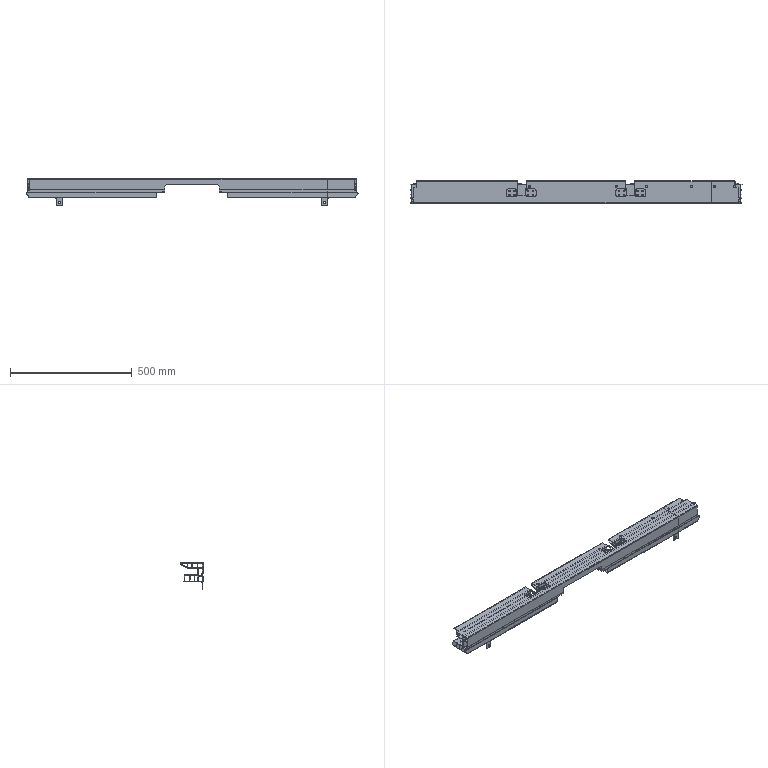NC program | NX | posted with a generic post | part box 1365 x 90.95 x 108.501 mm
Lines 9781 to 10665 of 25066:
(ZLEVEL_PROFILE_1_COPY_1_1 , TOOL : D8R0.5)
N19530 T08 M6
N19532 G54
N19534 G17 G0 G90 X660.495 Y57.439 B0. C0. S6000 M3
N19536 G43 Z30. H8
N19538 Z-42.865
N19540 G94 G1 Z-44.365 F1000.
N19542 X660.199 Y56.252
N19544 G3 X660.42 Y55.483 R0.8
N19546 G1 X660.758 Y55.156 F2500.
N19548 X662.222 Y53.696
N19550 X662.428 Y53.488
N19552 G3 X666.413 Y49.491 R729.531
N19554 G1 X666.616 Y49.475
N19556 Z-44.465
N19558 X666.413 Y49.491
N19560 G2 X663.219 Y52.689 R774.294
N19562 G1 X663.021 Y52.89
N19564 X660.715 Y55.202
N19566 X660.417 Y55.487
N19568 X660.418 Z-44.565
N19570 G2 X663.021 Y52.89 R195.375
N19572 G3 X666.414 Y49.491 R625.386
N19574 G1 X666.616 Y49.475
N19576 Z-44.665
N19578 X666.415 Y49.491
N19580 X665.211 Y50.69
N19582 X665.018 Y50.876
N19584 X664.809 Y51.09
N19586 X661.445 Y54.478
N19588 G3 X660.419 Y55.488 R64.335
N19590 G1 X660.42 Z-44.765
N19592 G2 X660.72 Y55.196 R23.551
N19594 X665.018 Y50.878 R530.21
N19596 G1 X665.214 Y50.69
N19598 X666.419 Y49.491
N19600 X666.616 Y49.475
N19602 Z-44.865
N19604 X666.425 Y49.491
N19606 X664.811 Y51.09
N19608 X664.619 Y51.282
N19610 G3 X663.021 Y52.891 R113.024
N19612 X661.024 Y54.894 R137.528
N19614 X660.421 Y55.489 R22.994
N19616 G1 X660.422 Y55.49 Z-44.965
N19618 G2 X661.024 Y54.899 R23.36
N19620 X663.021 Y52.892 R119.536
N19622 X664.619 Y51.286 R86.72
N19624 G1 X664.816 Y51.09
N19626 X666.431 Y49.491
N19628 X666.616 Y49.475
N19630 Z-45.064
N19632 X666.437 Y49.491
N19634 X666.217 Y49.713
N19636 X665.018 Y50.889
N19638 G3 X662.834 Y53.088 R301.433
N19640 X660.424 Y55.492 R93.733
N19642 G1 X660.442 Y55.478 Z-45.163
N19644 G2 X663.021 Y52.901 R125.339
N19646 X664.619 Y51.294 R58.969
N19648 G1 X664.824 Y51.09
N19650 X666.217 Y49.718
N19652 X666.443 Y49.491
N19654 X666.616 Y49.475
N19656 Z-45.262
N19658 X666.451 Y49.491
N19660 G3 X664.619 Y51.299 R214.938
N19662 X663.021 Y52.905 R42.782
N19664 X660.466 Y55.459 R115.023
N19666 G1 X660.504 Y55.426 Z-45.362
N19668 G2 X663.021 Y52.914 R106.424
N19670 X664.619 Y51.31 R47.085
N19672 G1 X666.463 Y49.491
N19674 X666.616 Y49.475
N19676 Z-45.462
N19678 X666.475 Y49.491
N19680 G3 X664.619 Y51.322 R957.072
N19682 X663.021 Y52.925 R54.744
N19684 X661.265 Y54.687 R80.824
N19686 G1 X660.547 Y55.392
N19688 X660.53 Y55.405
N19690 X660.554 Y55.39 Z-45.562
N19692 X660.869 Y55.087
N19694 X662.622 Y53.345
N19696 X663.021 Y52.936
N19698 G2 X664.862 Y51.09 R94.393
N19700 G1 X666.49 Y49.491
N19702 X666.616 Y49.475
N19704 Z-45.662
N19706 X666.508 Y49.491
N19708 G3 X664.872 Y51.09 R406.168
N19710 X660.587 Y55.368 R402.037
N19712 G1 X660.61 Y55.355 Z-45.762
N19714 G2 X665.285 Y50.69 R543.174
N19716 X666.525 Y49.491 R40.797
N19718 G1 X666.616 Y49.475
N19720 Z-45.862
N19722 X666.543 Y49.491
N19724 G3 X665.302 Y50.69 R40.86
N19726 G1 X664.895 Y51.09
N19728 G3 X663.299 Y52.689 R54.249
N19730 G1 X662.905 Y53.088
N19732 X660.747 Y55.232
N19734 X660.644 Y55.332
N19736 X660.674 Y55.313 Z-45.962
N19738 X664.529 Y51.49
N19740 X664.619 Y51.392
N19742 G3 X665.817 Y50.223 R29.773
N19744 G1 X666.56 Y49.491
N19746 X666.616 Y49.475
N19748 Z-46.062
N19750 X666.578 Y49.491
N19752 X665.817 Y50.239
N19754 G2 X664.619 Y51.411 R31.256
N19756 G1 X664.546 Y51.49
N19758 G2 X660.704 Y55.294 R6488.3
N19760 G1 X660.732 Y55.276 Z-46.162
N19762 X663.82 Y52.221
N19764 X664.563 Y51.49
N19766 G3 X665.779 Y50.291 R30.069
N19768 G1 X665.817 Y50.255
N19770 X666.595 Y49.491
N19772 X666.616 Y49.475
N19774 X667.016 Z-46.262
N19776 X666.616 Y49.488
N19778 X665.797 Y50.291
N19780 G2 X664.58 Y51.49 R32.969
N19782 X660.762 Y55.258 R1601.449
N19784 G1 X660.797 Y55.233 Z-46.362
N19786 G2 X665.418 Y50.67 R1621.061
N19788 G1 X666.64 Y49.491
N19790 X667.016 Y49.475
N19792 Z-46.462
N19794 X666.669 Y49.491
N19796 X665.415 Y50.69
N19798 G3 X660.823 Y55.217 R862.367
N19800 G1 X660.856 Y55.203 Z-46.562
N19802 G2 X665.442 Y50.69 R2264.451
N19804 G1 X666.699 Y49.491
N19806 X667.016 Y49.475
N19808 Z-46.662
N19810 X666.728 Y49.491
N19812 X665.418 Y50.741
N19814 G3 X660.888 Y55.188 R10000.
N19816 G1 X660.921 Y55.173 Z-46.762
N19818 X663.86 Y52.289
N19820 X664.219 Y51.946
N19822 G3 X666.758 Y49.491 R134.499
N19824 G1 X667.016 Y49.475
N19826 Z-46.862
N19828 X666.787 Y49.491
N19830 G2 X664.219 Y51.969 R138.511
N19832 G1 X663.879 Y52.289
N19834 X660.954 Y55.158
N19836 X660.987 Y55.144 Z-46.962
N19838 X661.024 Y55.109
N19840 X663.421 Y52.753
N19842 X663.898 Y52.289
N19844 G2 X664.723 Y51.49 R12.633
N19846 G1 X665.14 Y51.09
N19848 X666.817 Y49.491
N19850 X667.016 Y49.475
N19852 Z-47.062
N19854 X666.853 Y49.491
N19856 X665.167 Y51.09
N19858 X664.754 Y51.49
N19860 G3 X663.918 Y52.289 R13.176
N19862 G1 X663.421 Y52.772
N19864 X661.065 Y55.087
N19866 X661.02 Y55.13
N19868 X661.053 Y55.115 Z-47.162
N19870 G3 X664.377 Y51.889 R139.424
N19872 X666.89 Y49.491 R125.401
N19874 G1 X667.016 Y49.475
N19876 Z-47.262
N19878 X666.928 Y49.491
N19880 G2 X664.219 Y52.065 R139.113
N19882 X661.086 Y55.101 R170.902
N19884 G1 X661.119 Y55.088 Z-47.362
N19886 X661.224 Y54.985
N19888 X661.322 Y54.887
N19890 G3 X665.684 Y50.69 R374.935
N19892 G1 X665.817 Y50.553
N19894 G3 X666.217 Y50.195 R4.151
N19896 X666.973 Y49.491 R21.926
N19898 G1 X667.016 Y49.475
N19900 X667.415 Z-47.462
N19902 X667.018 Y49.491
N19904 X666.217 Y50.229
N19906 G2 X665.775 Y50.628 R2.857
N19908 G1 X665.72 Y50.69
N19910 G2 X661.152 Y55.072 R448.498
N19912 G1 X661.185 Y55.057 Z-47.562
N19914 X664.619 Y51.766
N19916 X665.326 Y51.09
N19918 X665.755 Y50.69
N19920 X665.817 Y50.618
N19922 X667.064 Y49.491
N19924 X667.415 Y49.475
N19926 Z-47.662
N19928 X667.111 Y49.491
N19930 X665.817 Y50.659
N19932 X665.36 Y51.09
N19934 X661.267 Y55.
N19936 X661.218 Y55.043
N19938 X661.257 Y55.034 Z-47.762
N19940 X665.394 Y51.09
N19942 X667.157 Y49.491
N19944 X667.415 Y49.475
N19946 Z-47.862
N19948 X667.204 Y49.491
N19950 X665.418 Y51.103
N19952 X664.619 Y51.855
N19954 X661.295 Y55.026
N19956 X661.334 Y55.018 Z-47.962
N19958 G3 X666.217 Y50.419 R200.946
N19960 X667.261 Y49.491 R51.744
N19962 G1 X667.415 Y49.475
N19964 Z-48.062
N19966 X667.321 Y49.491
N19968 X666.217 Y50.459
N19970 G2 X661.373 Y55.011 R204.666
N19972 G1 X661.412 Y55.003 Z-48.162
N19974 G3 X666.217 Y50.5 R208.729
N19976 G1 X667.381 Y49.491
N19978 X667.415 Y49.475
N19980 X667.466 Z-48.262
N19982 X666.217 Y50.546
N19984 G2 X661.451 Y54.995 R214.17
N19986 G1 X661.489 Y54.987 Z-48.362
N19988 G3 X666.217 Y50.591 R214.639
N19990 G1 X667.415 Y49.572
N19992 X667.526 Y49.475
N19994 X667.586 Z-48.462
N19996 G3 X666.217 Y50.637 R115.381
N19998 G2 X661.527 Y54.979 R213.984
N20000 G1 X661.566 Y54.971 Z-48.562
N20002 G3 X665.32 Y51.49 R210.792
N20004 G1 X665.418 Y51.398
N20006 G3 X667.415 Y49.685 R40.622
N20008 G1 X667.656 Y49.476
N20010 X667.666 Y49.475
N20012 X667.736 Z-48.662
N20014 G3 X667.216 Y49.891 R6.964
N20016 G2 X665.817 Y51.078 R195.276
N20018 X661.606 Y54.964 R235.459
N20020 G1 X661.645 Y54.956 Z-48.762
N20022 G3 X664.619 Y52.209 R191.352
N20024 G1 X665.018 Y51.845
N20026 G3 X667.815 Y49.474 R49.577
N20028 G1 X667.95 Y49.47 Z-48.795
N20030 X668.082 Y49.461 Z-48.828
N20032 X668.214 Y49.448 Z-48.862
N20034 X667.871 Y49.491
N20036 G2 X665.418 Y51.532 R48.127
N20038 G1 X665.014 Y51.889
N20040 X662.222 Y54.444
N20042 X661.684 Y54.949
N20044 X661.725 Y54.944 Z-48.962
N20046 G3 X665.571 Y51.45 R171.806
N20048 X667.949 Y49.491 R46.239
N20050 G1 X668.214 Y49.448
N20052 Z-49.062
N20054 X668.028 Y49.491
N20056 G2 X666.217 Y50.939 R69.157
N20058 X661.767 Y54.939 R168.722
N20060 G1 X661.81 Y54.935 Z-49.162
N20062 G3 X665.817 Y51.341 R150.74
N20064 G1 X666.026 Y51.156
N20066 G3 X666.801 Y50.512 R15.702
N20068 G1 X668.115 Y49.491
N20070 X668.214 Y49.448
N20072 X668.349 Y49.43 Z-49.195
N20074 X668.482 Y49.408 Z-49.228
N20076 X668.614 Y49.381 Z-49.262
N20078 X668.214 Y49.482
N20080 X666.645 Y50.692
N20082 G2 X666.122 Y51.124 R10.03
N20084 G1 X665.709 Y51.49
N20086 G2 X661.853 Y54.934 R132.391
N20088 G1 X661.897 Y54.933 Z-49.362
N20090 G3 X665.769 Y51.49 R122.516
N20092 X666.616 Y50.773 R11.575
N20094 G1 X668.214 Y49.551
N20096 X668.295 Y49.491
N20098 X668.614 Y49.381
N20100 Z-49.462
N20102 X668.39 Y49.491
N20104 G2 X666.297 Y51.09 R56.132
N20106 G1 X664.428 Y52.689
N20108 G3 X663.974 Y53.088 R4.546
N20110 G1 X663.82 Y53.225
N20112 X662.215 Y54.687
N20114 X661.942 Y54.932
N20116 G2 X661.693 Y55.692 R0.8
N20118 G1 X661.946 Y56.893
N20120 Z-47.962
N20122 G0 Z30.
N20124 X673.35 Y44.42
N20126 Z-42.865
N20128 G1 Z-44.365 F1000.
N20130 X672.15 Y43.727
N20132 G3 X671.75 Y43.034 R0.8
N20134 G1 X671.752 Y37.85 F2500.
N20136 X671.809 Y37.846
N20138 X672.758 Y37.838
N20140 G2 X675.059 Y37.528 R4.02
N20142 G3 X675.255 Y37.476 R0.604
N20144 G2 X678.751 Y33.504 R4.002
N20146 G1 X678.75 Y24.923
N20148 X678.74 Y24.91
N20150 G2 X678.75 Y24.556 R6.
N20152 G1 Y-30.121
N20154 G2 X677.555 Y-32.977 R4.004
N20156 G1 X676.189 Y-34.343
N20158 X668.418 Y-42.11
N20160 X668.379 Y-42.148 Z-44.465
N20162 X676.189 Y-34.343
N20164 X677.555 Y-32.976
N20166 G3 X678.75 Y-30.121 R4.004
N20168 G1 Y24.556
N20170 G3 X678.74 Y24.91 R6.
N20172 G1 X678.75 Y24.923
N20174 X678.751 Y33.504
N20176 G3 X675.247 Y37.477 R4.002
N20178 G1 X675.148 Y37.485
N20180 X675.059 Y37.528
N20182 G3 X672.758 Y37.838 R4.02
N20184 G1 X671.809 Y37.846
N20186 X671.752 Y37.85
N20188 X671.75 Y43.034
N20190 Z-44.565
N20192 X671.752 Y37.85
N20194 X671.809 Y37.846
N20196 X672.758 Y37.838
N20198 G2 X675.059 Y37.528 R4.02
N20200 G3 X675.255 Y37.476 R0.604
N20202 G2 X678.751 Y33.504 R4.002
N20204 G1 X678.75 Y24.923
N20206 X678.74 Y24.91
N20208 G2 X678.75 Y24.556 R6.
N20210 G1 Y-30.121
N20212 G2 X677.556 Y-32.976 R4.004
N20214 G1 X676.189 Y-34.343
N20216 X668.414 Y-42.118
N20218 X668.34 Y-42.186
N20220 X668.303 Y-42.225 Z-44.665
N20222 X676.189 Y-34.343
N20224 X677.556 Y-32.976
N20226 G3 X678.75 Y-30.121 R4.004
N20228 G1 Y24.556
N20230 G3 X678.74 Y24.91 R6.
N20232 G1 X678.75 Y24.923
N20234 X678.751 Y33.504
N20236 G3 X675.247 Y37.477 R4.002
N20238 G1 X675.148 Y37.485
N20240 X675.059 Y37.528
N20242 G3 X672.758 Y37.838 R4.02
N20244 G1 X671.809 Y37.846
N20246 X671.752 Y37.85
N20248 X671.75 Y43.034
N20250 Z-44.765
N20252 X671.753 Y37.85
N20254 X671.809 Y37.846
N20256 X672.758 Y37.838
N20258 G2 X675.059 Y37.528 R4.02
N20260 G3 X675.255 Y37.476 R0.604
N20262 G2 X678.751 Y33.504 R4.002
N20264 G1 X678.75 Y24.923
N20266 X678.74 Y24.91
N20268 G2 X678.75 Y24.556 R6.
N20270 G1 Y-30.121
N20272 G2 X677.556 Y-32.976 R4.004
N20274 G1 X676.189 Y-34.343
N20276 X668.263 Y-42.264
N20278 X668.223 Y-42.305 Z-44.865
N20280 X676.189 Y-34.343
N20282 X677.556 Y-32.976
N20284 G3 X678.75 Y-30.121 R4.004
N20286 G1 Y24.556
N20288 G3 X678.74 Y24.91 R6.
N20290 G1 X678.75 Y24.923
N20292 X678.751 Y33.504
N20294 G3 X675.247 Y37.477 R4.002
N20296 G1 X675.148 Y37.485
N20298 X675.059 Y37.528
N20300 G3 X672.758 Y37.838 R4.02
N20302 G1 X671.809 Y37.846
N20304 X671.765 Y37.85
N20306 Y39.499
N20308 X671.762 Y39.899
N20310 X671.752 Y39.975
N20312 Y42.443
N20314 X671.757 Y42.455
N20316 G2 X671.75 Y43.034 R8.354
N20318 G1 Z-44.965
N20320 X671.758 Y42.443
N20322 Y39.975
N20324 X671.774 Y39.899
N20326 G2 X671.78 Y37.85 R102.677
N20328 G1 X671.809 Y37.846
N20330 X672.758 Y37.838
N20332 G2 X675.059 Y37.528 R4.02
N20334 G3 X675.255 Y37.476 R0.604
N20336 G2 X678.751 Y33.504 R4.002
N20338 G1 X678.75 Y24.923
N20340 X678.74 Y24.91
N20342 G2 X678.75 Y24.556 R6.
N20344 G1 Y-30.121
N20346 G2 X677.556 Y-32.976 R4.004
N20348 G1 X676.189 Y-34.343
N20350 X668.196 Y-42.333
N20352 X668.172 Y-42.355 Z-45.064
N20354 X676.189 Y-34.343
N20356 X677.556 Y-32.976
N20358 G3 X678.75 Y-30.121 R4.004
N20360 G1 Y24.556
N20362 G3 X678.74 Y24.91 R6.
N20364 G1 X678.75 Y24.923
N20366 X678.751 Y33.504
N20368 G3 X675.247 Y37.477 R4.002
N20370 G1 X675.148 Y37.485
N20372 X675.059 Y37.528
N20374 G3 X672.758 Y37.838 R4.02
N20376 G1 X671.809 Y37.846
N20378 X671.796 Y37.85
N20380 G3 X671.79 Y39.899 R91.335
N20382 G1 X671.768 Y39.975
N20384 Y42.443
N20386 X671.774 Y42.455
N20388 X671.77 Y42.697
N20390 G2 X671.75 Y43.034 R1.744
N20392 G1 Z-45.163
N20394 G2 X671.782 Y42.593 R3.056
N20396 G1 Y39.975
N20398 X671.813 Y39.943
N20400 X671.811 Y39.899
N20402 G2 X671.813 Y37.85 R67.984
N20404 G1 X671.859 Y37.844
N20406 X672.758 Y37.838
N20408 G2 X675.059 Y37.528 R4.02
N20410 G3 X675.255 Y37.476 R0.604
N20412 G2 X678.751 Y33.504 R4.002
N20414 G1 X678.75 Y24.923
N20416 X678.74 Y24.91
N20418 G2 X678.75 Y24.556 R6.
N20420 G1 Y-30.121
N20422 G2 X677.556 Y-32.976 R4.004
N20424 G1 X676.189 Y-34.343
N20426 X668.214 Y-42.318
N20428 X668.149 Y-42.377
N20430 X668.127 Y-42.4 Z-45.262
N20432 X668.214 Y-42.318
N20434 X676.189 Y-34.343
N20436 X677.556 Y-32.975
N20438 G3 X678.75 Y-30.121 R4.004
N20440 G1 Y24.556
N20442 G3 X678.74 Y24.91 R6.
N20444 G1 X678.75 Y24.923
N20446 X678.751 Y33.504
N20448 G3 X675.255 Y37.476 R4.002
N20450 G1 X675.189 Y37.483
N20452 X675.141 Y37.482
N20454 X675.101 Y37.507
N20456 X675.005 Y37.552
N20458 G3 X672.848 Y37.85 R4.004
N20460 G1 X672.758 Y37.838
N20462 X672.358 Y37.841
N20464 X671.859 Y37.844
N20466 X671.838 Y37.85
N20468 G3 X671.837 Y39.899 R66.872
N20470 G1 X671.809 Y40.234
N20472 X671.8 Y40.299
N20474 Y42.584
N20476 G3 X671.75 Y43.131 R3.03
N20478 G1 Y43.271 Z-45.362
N20480 G2 X671.822 Y42.465 R4.138
N20482 G1 Y40.334
N20484 G2 X671.863 Y39.901 R2.833
N20486 X671.864 Y37.85 R62.188
N20488 G1 X671.909 Y37.844
N20490 X672.758 Y37.838
N20492 G2 X675.059 Y37.528 R4.02
N20494 G3 X675.255 Y37.476 R0.604
N20496 G2 X678.751 Y33.504 R4.002
N20498 G1 X678.75 Y24.923
N20500 X678.74 Y24.91
N20502 G2 X678.75 Y24.556 R6.
N20504 G1 Y-30.121
N20506 G2 X677.556 Y-32.975 R4.004
N20508 G1 X676.189 Y-34.343
N20510 X668.104 Y-42.424
N20512 X668.082 Y-42.447 Z-45.462
N20514 X676.189 Y-34.343
N20516 X677.557 Y-32.975
N20518 G3 X678.75 Y-30.121 R4.004
N20520 G1 Y24.556
N20522 G3 X678.74 Y24.91 R6.
N20524 G1 X678.75 Y24.923
N20526 X678.751 Y33.504
N20528 G3 X675.247 Y37.477 R4.002
N20530 G1 X675.148 Y37.485
N20532 X675.059 Y37.528
N20534 G3 X672.758 Y37.838 R4.02
N20536 G1 X672.009 Y37.844
N20538 X671.909
N20540 X671.894 Y37.85
N20542 X671.895 Y39.738
N20544 G3 X671.852 Y40.299 R3.609
N20546 G1 X671.87 Y40.309
N20548 X671.869 Y40.331
N20550 X671.849 Y40.338
N20552 Y42.475
N20554 G3 X671.75 Y43.359 R3.337
N20556 G1 Y43.496 Z-45.562
N20558 G2 X671.883 Y42.458 R3.712
N20560 G1 X671.88 Y42.297
N20562 Y40.343
N20564 X671.891 Y40.316
N20566 X671.923 Y39.899
N20568 X671.927 Y39.499
N20570 X671.928 Y37.85
N20572 X671.959 Y37.844
N20574 X672.758 Y37.838
N20576 G2 X675.059 Y37.528 R4.02
N20578 G3 X675.255 Y37.476 R0.604
N20580 G2 X678.751 Y33.504 R4.002
N20582 G1 X678.75 Y24.923
N20584 X678.74 Y24.91
N20586 G2 X678.75 Y24.556 R6.
N20588 G1 Y-30.121
N20590 G2 X677.557 Y-32.975 R4.004
N20592 G1 X676.189 Y-34.343
N20594 X668.058 Y-42.469
N20596 X668.035 Y-42.493 Z-45.662
N20598 X676.189 Y-34.343
N20600 X677.557 Y-32.975
N20602 G3 X678.75 Y-30.121 R4.004
N20604 G1 Y24.556
N20606 G3 X678.74 Y24.91 R6.
N20608 G1 X678.75 Y24.923
N20610 X678.751 Y33.504
N20612 G3 X675.247 Y37.477 R4.002
N20614 G1 X675.148 Y37.485
N20616 X675.059 Y37.528
N20618 G3 X672.758 Y37.838 R4.02
N20620 G1 X672.009 Y37.844
N20622 X671.965 Y37.85
N20624 X671.964 Y39.499
N20626 X671.961 Y39.899
N20628 X671.923 Y40.339
N20630 X671.916 Y40.359
N20632 Y42.475
N20634 G3 X671.75 Y43.631 R3.872
N20636 G1 Y43.751 Z-45.762
N20638 G2 X671.957 Y42.475 R3.936
N20640 G1 Y40.354
N20642 X671.978 Y40.329
N20644 X671.964 Y40.299
N20646 G2 X672.002 Y39.765 R3.895
N20648 G1 X672.003 Y37.85
N20650 X672.009 Y37.844
N20652 X672.059 Y37.843
N20654 X672.758 Y37.838
N20656 G2 X675.059 Y37.528 R4.02
N20658 G3 X675.255 Y37.476 R0.603
N20660 G2 X678.751 Y33.504 R4.002
N20662 G1 X678.75 Y24.923
N20664 X678.74 Y24.91
N20666 G2 X678.75 Y24.556 R6.
N20668 G1 Y-30.121
N20670 G2 X677.557 Y-32.975 R4.004
N20672 G1 X676.189 Y-34.343
N20674 X668.014 Y-42.518
N20676 X667.991 Y-42.538 Z-45.862
N20678 X676.189 Y-34.343
N20680 X677.557 Y-32.975
N20682 G3 X678.75 Y-30.121 R4.004
N20684 G1 Y24.556
N20686 G3 X678.74 Y24.91 R6.
N20688 G1 X678.75 Y24.923
N20690 X678.751 Y33.504
N20692 G3 X675.247 Y37.477 R4.002
N20694 G1 X675.148 Y37.485
N20696 X675.059 Y37.528
N20698 G3 X672.758 Y37.838 R4.02
N20700 G1 X672.059 Y37.843
N20702 X672.055 Y37.85
N20704 Y39.499
N20706 X672.051 Y39.899
N20708 X672.008 Y40.351
N20710 X672.003 Y40.362
N20712 Y42.475
N20714 G3 X671.75 Y43.873 R3.759
N20716 G1 Y44.007 Z-45.962
N20718 G2 X672.055 Y42.475 R3.945
N20720 G1 Y40.37
N20722 X672.069 Y40.299
N20724 X672.108 Y39.899
N20726 X672.109 Y37.843
N20728 X672.758 Y37.838
N20730 G2 X675.059 Y37.528 R4.02
N20732 G3 X675.255 Y37.476 R0.603
N20734 G2 X678.751 Y33.504 R4.002
N20736 G1 X678.75 Y24.923
N20738 X678.74 Y24.91
N20740 G2 X678.75 Y24.556 R6.
N20742 G1 Y-30.121
N20744 G2 X677.565 Y-32.967 R4.002
N20746 G1 X676.189 Y-34.343
N20748 X668.014 Y-42.518
N20750 X667.968 Y-42.559
N20752 X667.945 Y-42.581 Z-46.062
N20754 X668.014 Y-42.518
N20756 X676.189 Y-34.343
N20758 X677.565 Y-32.967
N20760 G3 X678.75 Y-30.121 R4.001
N20762 G1 Y24.556
N20764 G3 X678.74 Y24.91 R6.
N20766 G1 X678.75 Y24.923
N20768 X678.751 Y33.511
N20770 G3 X675.447 Y37.443 R3.991
N20772 G1 X675.115 Y37.501
N20774 G3 X673.008 Y37.869 R3.982
N20776 G1 X672.958 Y37.864
N20778 X672.808 Y37.846
N20780 X672.73 Y37.841
N20782 X672.259
N20784 X672.209 Y37.843
N20786 X672.163 Y37.85
N20788 G3 X672.162 Y39.886 R59.674
N20790 X672.112 Y40.367 R2.872
N20792 G1 Y42.475
N20794 G3 X671.75 Y44.13 R3.828
N20796 G1 Y44.256 Z-46.162
N20798 G2 X672.176 Y42.475 R3.711
N20800 G1 Y40.377
N20802 X672.184 Y40.36
N20804 X672.224 Y39.899
N20806 X672.23 Y37.85
N20808 X672.239 Y37.835
N20810 X672.255 Y37.842
N20812 X672.758 Y37.838
N20814 X672.848 Y37.85
N20816 G2 X675.005 Y37.552 R4.003
N20818 G1 X675.1 Y37.508
N20820 X675.141 Y37.482
N20822 X675.189 Y37.483
N20824 X675.255 Y37.476
N20826 G2 X678.751 Y33.504 R4.002
N20828 G1 X678.75 Y24.923
N20830 X678.74 Y24.91
N20832 G2 X678.75 Y24.556 R6.
N20834 G1 Y-30.121
N20836 G2 X677.565 Y-32.967 R4.001
N20838 G1 X676.189 Y-34.343
N20840 X668.014 Y-42.518
N20842 X667.923 Y-42.603
N20844 X667.902 Y-42.626 Z-46.262
N20846 X676.189 Y-34.343
N20848 X677.565 Y-32.967
N20850 G3 X678.75 Y-30.121 R4.001
N20852 G1 Y24.556
N20854 G3 X678.74 Y24.91 R6.
N20856 G1 X678.75 Y24.923
N20858 X678.751 Y33.504
N20860 G3 X675.255 Y37.476 R4.002
N20862 G1 X675.189 Y37.483
N20864 X675.141 Y37.482
N20866 X675.1 Y37.508
N20868 X675.005 Y37.552
N20870 G3 X672.848 Y37.85 R4.003
N20872 G1 X672.758 Y37.838
N20874 X672.358 Y37.841
N20876 X672.309
N20878 X672.301 Y37.85
N20880 G3 X672.298 Y39.899 R63.582
N20882 G1 X672.262 Y40.332
N20884 X672.247 Y40.382
N20886 Y42.475
N20888 G3 X671.75 Y44.397 R3.764
N20890 G1 Y44.526 Z-46.362
N20892 G2 X672.326 Y42.475 R3.743
N20894 G1 Y40.346
N20896 X672.344 Y40.299
N20898 X672.372 Y39.899
N20900 G2 X672.374 Y37.85 R51.771
N20902 G1 X672.408 Y37.84
N20904 X672.681
N20906 X672.767 Y37.832
N20908 X672.852 Y37.851
N20910 G2 X675.005 Y37.552 R4.007
N20912 G1 X675.1 Y37.508
N20914 X675.141 Y37.482
N20916 X675.189 Y37.483
N20918 X675.255 Y37.476
N20920 G2 X678.751 Y33.504 R4.002
N20922 G1 X678.75 Y24.923
N20924 X678.74 Y24.91
N20926 G2 X678.75 Y24.556 R6.
N20928 G1 Y-30.121
N20930 G2 X677.565 Y-32.967 R4.001
N20932 G1 X676.189 Y-34.343
N20934 X667.88 Y-42.649
N20936 X667.856 Y-42.671 Z-46.462
N20938 X676.189 Y-34.343
N20940 X677.565 Y-32.967
N20942 G3 X678.75 Y-30.121 R4.001
N20944 G1 Y24.556
N20946 G3 X678.74 Y24.91 R6.
N20948 G1 X678.75 Y24.923
N20950 X678.751 Y33.504
N20952 G3 X675.255 Y37.476 R4.002
N20954 G1 X675.189 Y37.483
N20956 X675.141 Y37.482
N20958 X675.1 Y37.508
N20960 X675.005 Y37.552
N20962 G3 X672.958 Y37.864 R4.009
N20964 G1 X672.858 Y37.852
N20966 G2 X672.458 Y37.84 R2.323
N20968 G3 X672.454 Y39.899 R46.354
N20970 G1 X672.423 Y40.299
N20972 X672.414 Y40.336
N20974 Y42.475
N20976 G3 X671.75 Y44.649 R3.699
N20978 G1 Y44.792 Z-46.562
N20980 G2 X672.511 Y42.475 R3.813
N20982 G1 Y39.975
N20984 X672.543 Y39.899
N20986 G2 X672.546 Y37.856 R41.562
N20988 G1 X672.544 Y37.844
N20990 X672.556 Y37.843
N20992 G3 X672.848 Y37.85 R0.936
N20994 G2 X675.005 Y37.552 R4.003
N20996 G1 X675.1 Y37.508
N20998 X675.141 Y37.482
N21000 X675.189 Y37.483
N21002 X675.255 Y37.476
N21004 G2 X678.751 Y33.504 R4.002
N21006 G1 X678.75 Y24.923
N21008 X678.74 Y24.91
N21010 G2 X678.75 Y24.556 R6.
N21012 G1 Y-30.121
N21014 G2 X677.565 Y-32.966 R4.001
N21016 G1 X676.189 Y-34.343
N21018 X667.833 Y-42.694
N21020 X667.813 Y-42.719 Z-46.662
N21022 X676.189 Y-34.343
N21024 X677.565 Y-32.966
N21026 G3 X678.75 Y-30.121 R4.001
N21028 G1 Y24.556
N21030 G3 X678.74 Y24.91 R6.
N21032 G1 X678.75 Y24.923
N21034 X678.751 Y33.504
N21036 G3 X675.255 Y37.477 R4.002
N21038 G1 X675.186 Y37.484
N21040 X675.141 Y37.482
N21042 X675.103 Y37.507
N21044 X675.005 Y37.552
N21046 G3 X672.748 Y37.836 R4.02
N21048 G1 X672.69 Y37.825
N21050 X672.636 Y37.85
N21052 G3 X672.617 Y40.101 R26.796
N21054 G1 Y42.475
N21056 G3 X671.75 Y44.918 R3.889
N21058 G1 Y45.037 Z-46.762
N21060 G2 X672.717 Y42.475 R3.888
N21062 G1 Y40.091
N21064 G2 X672.734 Y37.85 R28.569
N21066 G1 X672.758 Y37.838
N21068 G2 X675.005 Y37.552 R4.02
N21070 G1 X675.103 Y37.507
N21072 X675.141 Y37.482
N21074 X675.186 Y37.484
N21076 X675.255 Y37.477
N21078 G2 X678.751 Y33.504 R4.003
N21080 G1 X678.75 Y24.923
N21082 X678.74 Y24.91
N21084 G2 X678.75 Y24.556 R6.
N21086 G1 Y-30.121
N21088 G2 X677.566 Y-32.966 R4.001
N21090 G1 X676.189 Y-34.343
N21092 X667.793 Y-42.736
N21094 X667.774 Y-42.753 Z-46.862
N21096 X676.189 Y-34.343
N21098 X677.566 Y-32.966
N21100 G3 X678.75 Y-30.121 R4.001
N21102 G1 Y24.556
N21104 G3 X678.74 Y24.91 R6.
N21106 G1 X678.75 Y24.923
N21108 X678.751 Y33.504
N21110 G3 X675.247 Y37.477 R4.003
N21112 G1 X675.149 Y37.485
N21114 X675.059 Y37.528
N21116 G3 X672.833 Y37.85 R4.038
N21118 X672.817 Y40.081 R30.886
N21120 G1 Y42.475
N21122 G3 X671.75 Y45.149 R3.909
N21124 G1 Y45.251 Z-46.962
N21126 G2 X672.917 Y42.475 R3.907
N21128 G1 Y40.071
N21130 G2 X672.932 Y37.901 R32.744
N21132 G1 X672.928 Y37.877
N21134 X672.947 Y37.86
N21136 X672.971 Y37.865
N21138 G2 X675.115 Y37.501 R3.982
N21140 G1 X675.445 Y37.443
N21142 G2 X678.751 Y33.511 R3.991
N21144 G1 X678.75 Y24.923
N21146 X678.74 Y24.91
N21148 G2 X678.75 Y24.556 R6.
N21150 G1 Y-30.121
N21152 G2 X677.566 Y-32.966 R4.001
N21154 G1 X676.189 Y-34.343
N21156 X667.756 Y-42.771
N21158 X667.737 Y-42.789 Z-47.062
N21160 X667.815 Y-42.717
N21162 X676.189 Y-34.343
N21164 X677.566 Y-32.966
N21166 G3 X678.75 Y-30.121 R4.001
N21168 G1 Y24.556
N21170 G3 X678.74 Y24.91 R6.
N21172 G1 X678.75 Y24.923
N21174 X678.751 Y33.511
N21176 G3 X675.445 Y37.443 R3.991
N21178 G1 X675.115 Y37.501
N21180 G3 X673.621 Y37.875 R3.817
N21182 G1 X673.03 Y37.9
N21184 G3 X673.017 Y40.064 R35.391
N21186 G1 Y42.475
N21188 G3 X671.75 Y45.348 R3.919
N21190 G1 Y45.436 Z-47.162
N21192 G2 X673.117 Y42.475 R3.92
N21194 G1 Y40.046
N21196 G2 X673.129 Y37.9 R37.902
N21198 G1 X673.636 Y37.876
N21200 G2 X675.115 Y37.501 R3.843
N21202 G1 X675.445 Y37.443
N21204 G2 X678.751 Y33.511 R3.991
N21206 G1 X678.75 Y24.923
N21208 X678.74 Y24.91
N21210 G2 X678.75 Y24.556 R6.
N21212 G1 Y-30.121
N21214 G2 X677.566 Y-32.966 R4.001
N21216 G1 X676.189 Y-34.343
N21218 X667.719 Y-42.808
N21220 X667.701 Y-42.827 Z-47.262
N21222 X676.189 Y-34.343
N21224 X677.566 Y-32.966
N21226 G3 X678.75 Y-30.121 R4.001
N21228 G1 Y24.556
N21230 G3 X678.74 Y24.91 R6.
N21232 G1 X678.75 Y24.923
N21234 X678.751 Y33.511
N21236 G3 X675.444 Y37.443 R3.991
N21238 G1 X675.115 Y37.501
N21240 G3 X673.659 Y37.876 R3.874
N21242 G1 X673.227 Y37.9
N21244 G3 X673.217 Y40.028 R40.959
N21246 G1 Y42.475
N21248 G3 X671.75 Y45.521 R3.925
N21250 G1 X671.748 Y45.6 Z-47.362
N21252 G2 X673.317 Y42.475 R3.931
N21254 G1 Y40.01
N21256 X673.325 Y39.899
N21258 X673.326 Y37.9
N21260 X673.407 Y37.889
N21262 X673.65 Y37.876
N21264 G2 X675.115 Y37.501 R3.862
N21266 G1 X675.444 Y37.444
N21268 G2 X678.751 Y33.511 R3.991
N21270 G1 X678.75 Y24.923
N21272 X678.74 Y24.91
N21274 G2 X678.75 Y24.556 R6.
N21276 G1 Y-30.121
N21278 G2 X677.566 Y-32.966 R4.001
N21280 G1 X676.189 Y-34.343
N21282 X667.688 Y-42.842
N21284 X667.676 Y-42.852 Z-47.462
N21286 X676.189 Y-34.343
N21288 X677.566 Y-32.965
N21290 G3 X678.75 Y-30.121 R4.001
N21292 G1 Y24.556